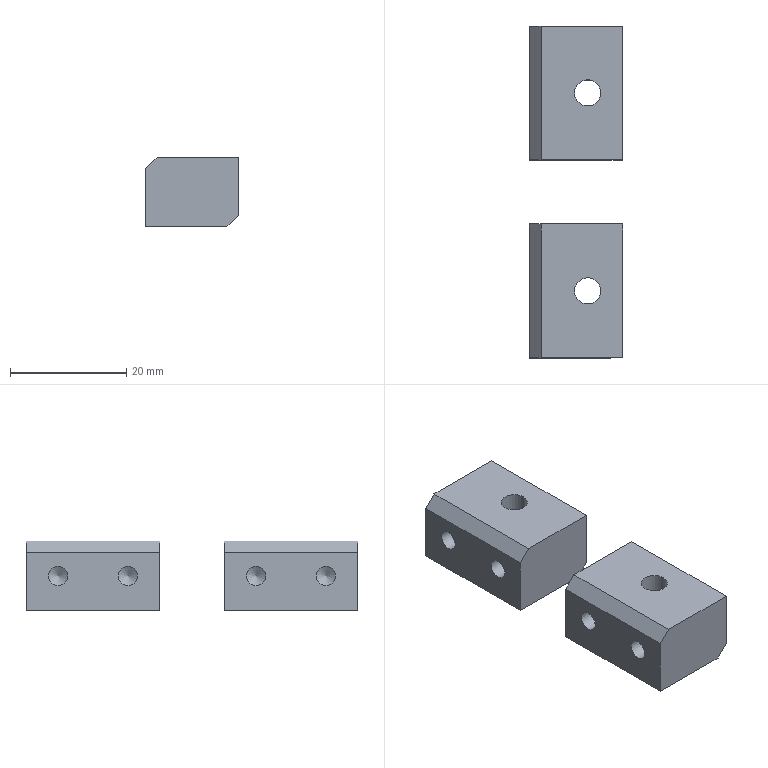CAM job | NX | 3+2 milling, drilling | part box 16 x 57 x 12 mm | stock box 20 x 62 x 15 mm
Tools:
number,name,description,diameter,corner_radius,flute_length,length,flutes
9,D10,平底铣刀-粗,10.0,0.0,35.0,75.0,2
10,D10-J,平底铣刀-精,10.0,0.0,35.0,75.0,2
1,D80R0.8飞刀,圆鼻刀-粗,80.0,0.8,50.0,75.0,2
2,D6倒角刀,倒角刀,6.0,0.0,3.0,25.0,2
21,M4X0.7,丝锥,3.3,0.0,35.0,50.0,2
13,钻头3.3,Twist Drill 3.3 mm,3.3,0.0,35.0,35.008,2
Operations:
program,operation,operation_type,tool,method,geometry_group,spindle_rpm,surface_speed,feed_per_tooth,feed_cut,feed_plunge,cut_length_mm,path_length_mm,cut_time_min,machine_time_min
A,TOP_FACE_ROUGHING,FaceMilling,D80R0.8飞刀,LAYERED_ROUGHING-DEPTH_K-STEPOVER_G,W-A,4000.0,1005.31,0.375,3000.0,100.0,151.0,186.8,0.0503,0.0539
A,TOP_FACE,FaceMilling,D80R0.8飞刀,SIDE_EDGE_FINISHING-DEPTH_K-STEPOVER_G,W-A,4000.0,1005.31,0.125,1000.0,100.0,151.0,187.0,0.151,0.1546
A,Z_LEVEL_HELICAL_ROUGHING-MEDIUM_COPY,ZLevelMilling,D10,LAYERED_ROUGHING-DEPTH_K-STEPOVER_G,W-A,8000.0,251.32,0.25,4000.0,100.0,5790.341,5932.568,1.448,1.462
A,Z_LEVEL_FINISHING_ZIGZAG_CLIMB_COPY,ZLevelMilling,D10,Z_LEVEL_CLIMB_FACE-DEPTH_K-STEPOVER_G,W-A,7000.0,219.911,0.3214,4500.0,100.0,778.511,893.356,0.173,0.1845
A,SPOT_DRILL-DEPTH_0.8,Operation,D6倒角刀,NONE,W-A,8000.0,150.796,0.0312,500.0,90.0,7.2,103.506,0.0144,0.024
A,BLIND_CONE_HOLE-M4_TAP_DRILL,Operation,钻头3.3,NONE,W-A,3000.0,31.102,0.02,120.0,90.0,40.366,169.837,0.3364,0.3493
A,SELECTED_SOLIDS_ONLY,SurfaceContour,D6倒角刀,METHOD,W-A,8000.0,150.796,0.1875,3000.0,100.0,113.799,241.475,0.0379,0.0507
A,DRILL_CHAMFER_1,Operation,D6倒角刀,METHOD,W-A,8000.0,150.796,0.0312,500.0,0.0,20.8,137.542,0.0416,0.0533
A,BLIND_CONE_HOLE-M4_TAPPING,Operation,M4X0.7,METHOD,W-A,800.0,8.294,0.0004,0.7,90.0,28.4,145.906,40.571,40.583
A,PLANAR_DEBURR_6X45L_COPY,SurfaceContour,D6倒角刀,CLIMB_FACE_CHAMFER-DEPTH_0-STEPOVER_G,W-A,6500.0,122.519,0.1154,1500.0,100.0,133.662,385.573,0.0891,0.1143
A,FLOOR_WALL_MILL_CHAMFER_COPY,VolumeBased25DMillingOperation,D6倒角刀,CLIMB_FACE_CHAMFER-DEPTH_0-STEPOVER_G,W-A,6500.0,122.519,0.1154,1500.0,100.0,69.03,157.03,0.046,0.0548
A,Z_LEVEL_FINISHING-MEDIUM_COPY,ZLevelMilling,D10-J,SIDE_EDGE_FINISHING-DEPTH_K-STEPOVER_G,W-A,6000.0,188.496,0.0833,1000.0,100.0,433.419,608.971,0.4334,0.451